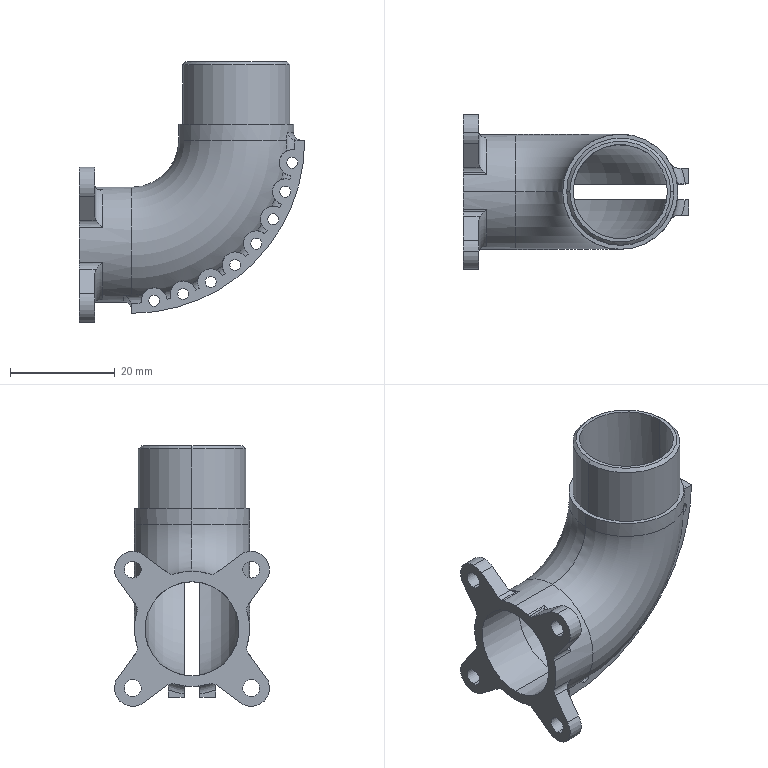Part | SolidWorks | features ICE 15, Fillet 6, Chamfer 5, MirrorPattern 3, RevCut 1, Revolution 1 | 1 solid | 150 faces | box 43.074 x 29.627 x 49.814 mm | volume 7359 mm3 | cylinder 92 | torus 31 | plane 25 | cone 2 | commonest cylinder face diameters 2.1 x32 5 x24 3 x10 3.2 x8 7 x6 18 x4